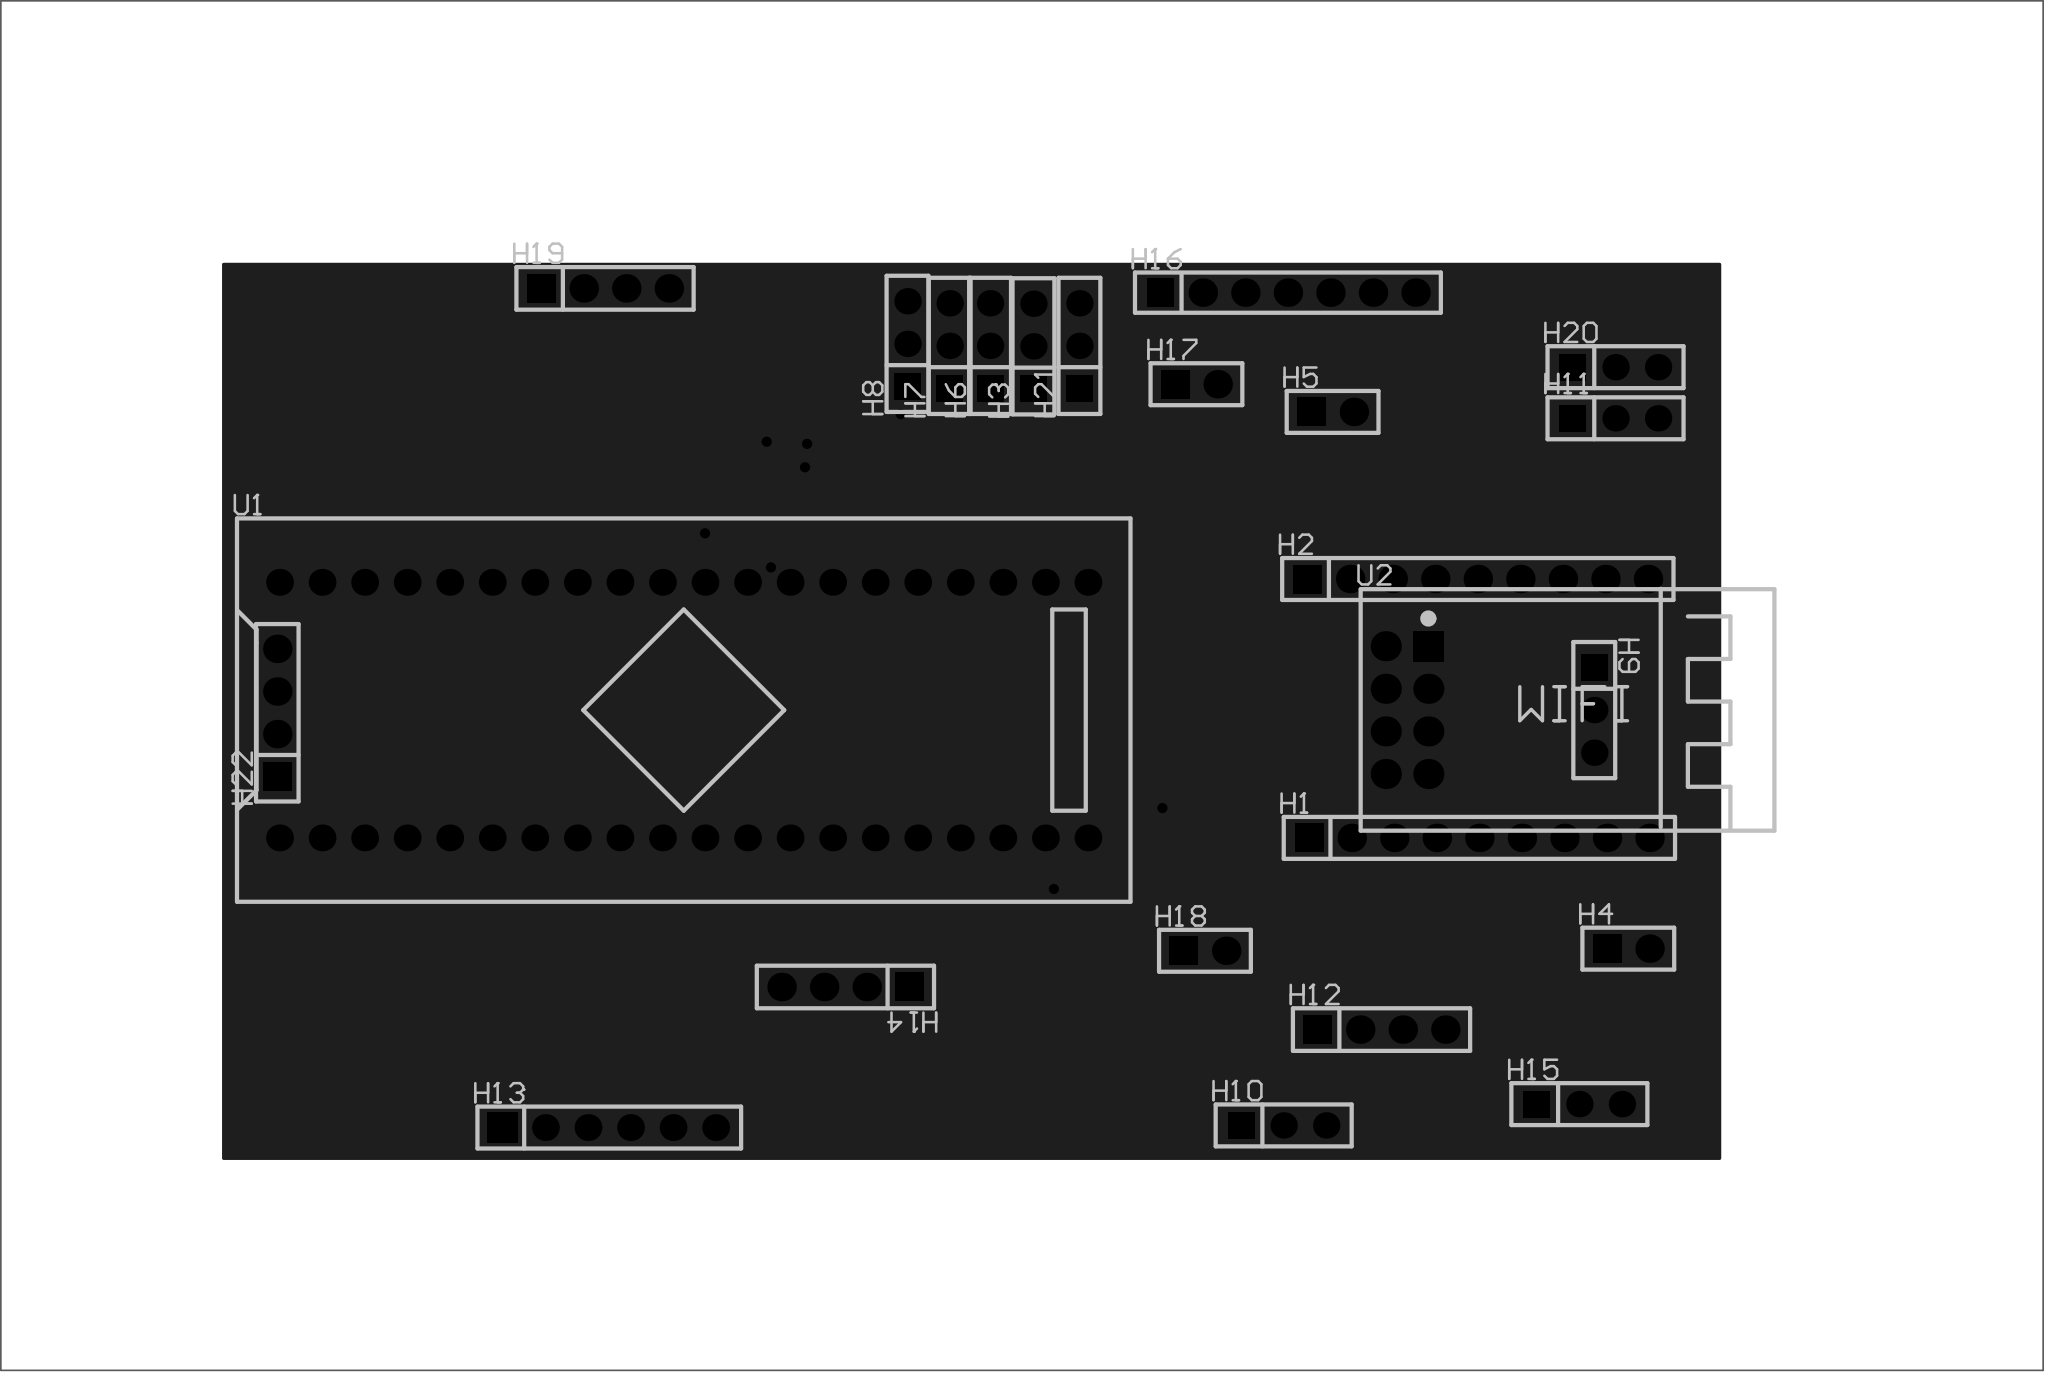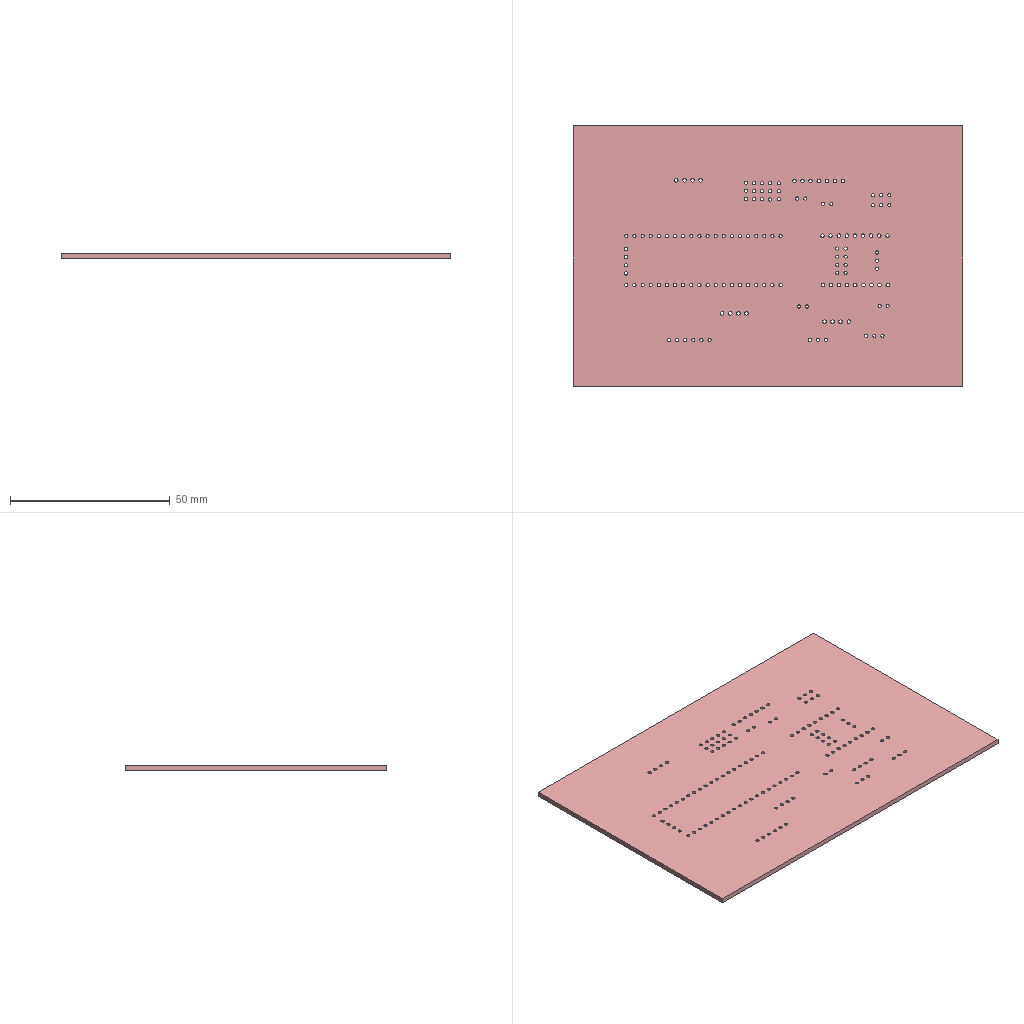Circuit board layout | Altium Designer | box 121.9 x 81.7 x 1.6 mm
Layer stack:
# Altium Designer layer stack of  (unit mm; dielectric type: 0 none, 1 core, 2 prepreg, 3 surface material)
index,name,kind,layer,copper_thickness_mm,dielectric_type,dielectric_thickness_mm,dielectric_material,dielectric_constant
0,Top Paste Mask Layer,other,,,,,,
1,Top Silkscreen Layer,other,,,,,,
2,Top Solder Mask Layer,dielectric,,,3,0.01,,3.3
3,Top Layer,copper,Top Layer,0.035,,,,
4,Dielectric1,dielectric,,,3,1.51,FR4,4.5
5,Bottom Layer,copper,Bottom Layer,0.035,,,,
6,Bottom Solder Mask Layer,dielectric,,,3,0.01,,3.3
7,Bottom Silkscreen Layer,other,,,,,,
8,Bottom Paste Mask Layer,other,,,,,,
# drill layer pairs: low layer,high layer
drill_pair,Top Layer,Bottom Layer
Part placement:
Designator,Comment,Layer,Footprint,Center-X(mm),Center-Y(mm),Rotation
H1,,TopLayer,HDR-TH_9P-P2.54-V-F-1,158.115,101.6,0
H2,,TopLayer,HDR-TH_9P-P2.54-V-F-1,158.022,117.036,0
H3,,TopLayer,HDR-TH_3P-P2.54-V-F,131.494,130.91,90
H4,,TopLayer,HDR-TH_2P-P2.54-V-F,167.005,94.996,0
H7,,TopLayer,HDR-TH_3P-P2.54-V-F,126.492,130.937,90
H18,,TopLayer,HDR-TH_2P-P2.54-V-F,141.732,94.869,0
H19,,TopLayer,HDR-TH_4P-P2.54-V-F,105.918,134.366,0
H20,,TopLayer,HDR-TH_3P-P2.54-V-F,166.243,129.667,0
H21,,TopLayer,HDR-TH_3P-P2.54-V-F,134.239,130.937,90
H22,,TopLayer,HDR-TH_4P-P2.54-V-F,86.353,109.06,90
U2,Ai-Thinker ESP-01S ESP8266,TopLayer,WIFIM-TH_8P-L24.7-W14.4-P2.54,153.797,109.22,0
H5,,TopLayer,HDR-TH_2P-P2.54-V-F,149.352,127,0
H6,,TopLayer,HDR-TH_3P-P2.54-V-F,128.905,130.937,90
H8,,TopLayer,HDR-TH_3P-P2.54-V-F,123.976,131.058,90
H9,,TopLayer,HDR-TH_3P-P2.54-V-F,164.973,109.22,270
H10,,TopLayer,HDR-TH_3P-P2.54-V-F,146.431,84.455,0
H11,,TopLayer,HDR-TH_3P-P2.54-V-F,166.243,126.619,0
H12,,TopLayer,HDR-TH_4P-P2.54-V-F,152.273,90.17,0
H13,,TopLayer,HDR-TH_6P-P2.54-V-F,106.172,84.328,0
H14,,TopLayer,HDR-TH_4P-P2.54-V-F,120.269,92.71,180
H15,,TopLayer,HDR-TH_3P-P2.54-V-F,164.084,85.725,0
H16,,TopLayer,HDR-TH_7P-P2.54-V-F,146.685,134.112,0
H17,,TopLayer,HDR-TH_2P-P2.54-V-F,141.224,128.651,0
U1,STM32F103C8T6-Card,TopLayer,CONN-TH_L53.3-W22.9_STM32F103C8T6-CARD,110.617,109.22,0
Pad and via stacks:
# Altium Designer via and pad stacks of  (unit mm). Each distinct definition once, with the count of objects using it.
# via: kind,start_layer,end_layer,hole_mm,diameter_mm,mode(0 simple;1 top-mid-bottom;2 full stack),diameter_per_layer,count,example_net
# pad: kind,layer,hole_mm,hole_type(0 round;1 square;2 slot),plating,top_size,top_shape(1 round;2 rect;3 octagon;9 rounded rect),mid_size,bottom_size,mode,footprint,size_per_layer,count,example
pad,Multi-Layer,1.1,0,plated,1.7x1.7,2,1.7x1.7,1.7x1.7,0,HDR-TH_9P-P2.54-V-F-1,,2,H1.1
pad,Multi-Layer,1.1,0,plated,1.7x1.7,1,1.7x1.7,1.7x1.7,0,HDR-TH_9P-P2.54-V-F-1,,16,H1.2
pad,Multi-Layer,1.02,0,plated,1.575x1.575,1,1.575x1.575,1.575x1.575,0,HDR-TH_3P-P2.54-V-F,,20,H3.3
pad,Multi-Layer,1.02,0,plated,1.575x1.575,2,1.575x1.575,1.575x1.575,0,HDR-TH_3P-P2.54-V-F,,10,H3.1
pad,Multi-Layer,1,0,plated,1.7x1.7,2,1.7x1.7,1.7x1.7,0,HDR-TH_2P-P2.54-V-F,,4,H4.1
pad,Multi-Layer,1,0,plated,1.7x1.7,1,1.7x1.7,1.7x1.7,0,HDR-TH_2P-P2.54-V-F,,4,H4.2
pad,Multi-Layer,1.1,0,plated,1.7x1.7,2,1.7x1.7,1.7x1.7,0,HDR-TH_4P-P2.54-V-F,,4,H19.1
pad,Multi-Layer,1.1,0,plated,1.7x1.7,1,1.7x1.7,1.7x1.7,0,HDR-TH_4P-P2.54-V-F,,12,H19.2
pad,Multi-Layer,1,0,plated,1.8x1.8,1,1.8x1.8,1.8x1.8,0,WIFIM-TH_8P-L24.7-W14.4-P2.54,,7,U2.8
pad,Multi-Layer,1,0,plated,1.8x1.8,2,1.8x1.8,1.8x1.8,0,WIFIM-TH_8P-L24.7-W14.4-P2.54,,1,U2.1
pad,Multi-Layer,1.02,0,plated,1.6x1.6,1,1.6x1.6,1.6x1.6,0,HDR-TH_6P-P2.54-V-F,,5,H13.6
pad,Multi-Layer,1.02,0,plated,1.8x1.8,2,1.8x1.8,1.8x1.8,0,HDR-TH_6P-P2.54-V-F,,1,H13.1
pad,Multi-Layer,1.1,0,plated,1.7x1.7,1,1.7x1.7,1.7x1.7,0,HDR-TH_7P-P2.54-V-F,,6,H16.7
pad,Multi-Layer,1.1,0,plated,1.575x1.7,2,1.575x1.7,1.575x1.7,0,HDR-TH_7P-P2.54-V-F,,1,H16.1
pad,Multi-Layer,1,0,plated,1.6x1.6,1,1.6x1.6,1.6x1.6,0,CONN-TH_L53.3-W22.9_STM32F103C8T6-CARD,,40,U1.1
via,Top Layer,Bottom Layer,0.3048,0.61,0,,8,PA6
Copper pours:
name,layer,net,type(0 solid;1 hatched;2 none)
Top Layer-GND,Top Layer,GND,0
Bottom Layer-GND,Bottom Layer,GND,0
Design rules, without the lines most boards share:
# Altium Designer design rules of  (exported by Altium Designer, unit mm)
# columns: name | kind | enabled | priority | scope1 | scope2 | descriptor | typed fields (field=value)
copperThickness1oz_2 | 2 | enabled | 2 | All | All | Width Constraint (Min=5mil) (Max=100mil) (Preferred=30mil) (All) |